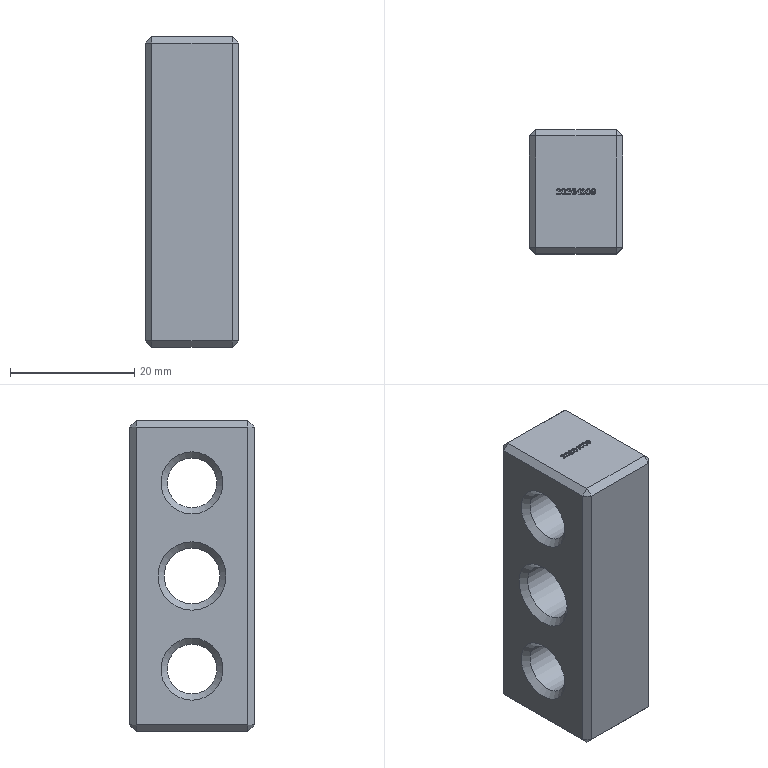Part | NX | features BREP 8, solid 2, CHAMFER 1, SUBTRACT 1 | 1 solid | 92 faces | box 15 x 20 x 50 mm | volume 12288 mm3 | spline 44 | plane 39 | cone 6 | cylinder 3 | commonest cylinder face diameters 8 x2 9 x1